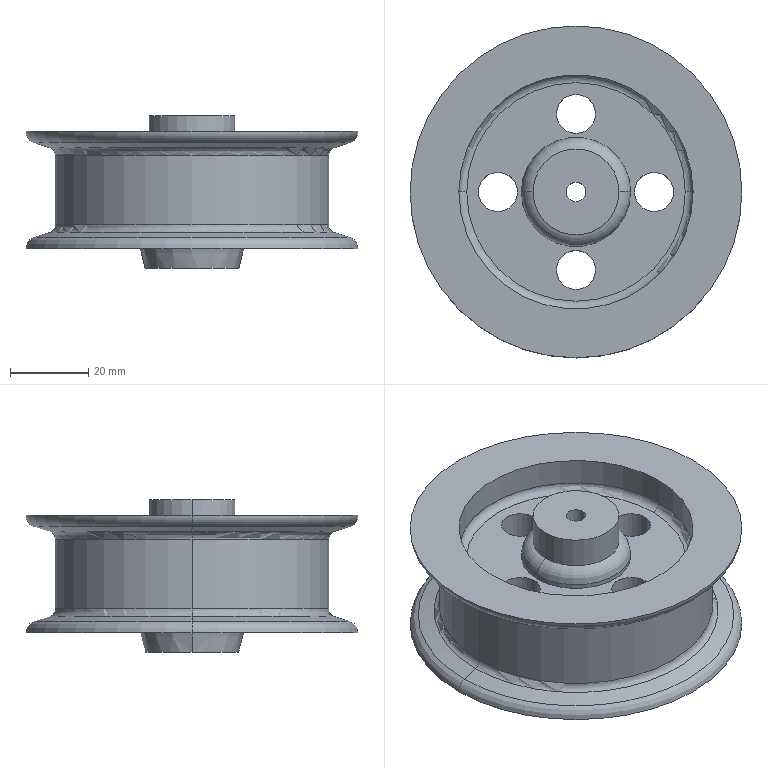Part | SolidWorks | features ICE 6, Fillet 2, Blend 1, Chamfer 1, Extrusion 1, HoleWzd 1, RevCut 1 | 1 solid | 46 faces | box 85 x 85 x 39 mm | volume 97267 mm3 | cylinder 20 | torus 12 | cone 8 | plane 6 | commonest cylinder face diameters 10 x8 60 x4 5 x2 22 x2 28 x2 70 x2
STEP:
#1=CARTESIAN_POINT('',(-12.,0.,-20.));
#2=VERTEX_POINT('',#1);
#3=CARTESIAN_POINT('',(12.,0.,-20.));
#4=VERTEX_POINT('',#3);
#5=CARTESIAN_POINT('',(0.,0.,-20.));
#6=DIRECTION('',(0.,0.,-1.));
#7=DIRECTION('',(-1.,0.,0.));
#8=AXIS2_PLACEMENT_3D('',#5,#6,#7);
#9=CIRCLE('',#8,12.);
#10=EDGE_CURVE('',#2,#4,#9,.T.);
#11=ORIENTED_EDGE('',*,*,#10,.F.);
#12=CARTESIAN_POINT('',(-14.,0.,-12.));
#13=VERTEX_POINT('',#12);
#14=CARTESIAN_POINT('',(-12.,0.,-20.));
#15=DIRECTION('',(-0.2425,0.,0.9701));
#16=VECTOR('',#15,1000.);
#17=LINE('',#14,#16);
#18=EDGE_CURVE('',#2,#13,#17,.T.);
#19=ORIENTED_EDGE('',*,*,#18,.T.);
#20=CARTESIAN_POINT('',(14.,0.,-12.));
#21=VERTEX_POINT('',#20);
#22=CARTESIAN_POINT('',(0.,0.,-12.));
#23=DIRECTION('',(0.,0.,-1.));
#24=DIRECTION('',(-1.,0.,0.));
#25=AXIS2_PLACEMENT_3D('',#22,#23,#24);
#26=CIRCLE('',#25,14.);
#27=EDGE_CURVE('',#13,#21,#26,.T.);
#28=ORIENTED_EDGE('',*,*,#27,.T.);
#29=CARTESIAN_POINT('',(12.,0.,-20.));
#30=DIRECTION('',(0.2425,0.,0.9701));
#31=VECTOR('',#30,1000.);
#32=LINE('',#29,#31);
#33=EDGE_CURVE('',#4,#21,#32,.T.);
#34=ORIENTED_EDGE('',*,*,#33,.F.);
#35=EDGE_LOOP('',(#11,#19,#28,#34));
#36=FACE_OUTER_BOUND('',#35,.T.);
#37=CARTESIAN_POINT('',(0.,0.,-20.));
#38=DIRECTION('',(0.,0.,1.));
#39=DIRECTION('',(1.,0.,0.));
#40=AXIS2_PLACEMENT_3D('',#37,#38,#39);
#41=CONICAL_SURFACE('',#40,12.,0.245);
#42=ADVANCED_FACE('',(#36),#41,.T.);
#43=CARTESIAN_POINT('',(2.5,0.,-20.));
#44=VERTEX_POINT('',#43);
#45=CARTESIAN_POINT('',(-2.5,0.,-20.));
#46=VERTEX_POINT('',#45);
#47=CARTESIAN_POINT('',(0.,0.,-20.));
#48=DIRECTION('',(0.,0.,-1.));
#49=DIRECTION('',(-1.,0.,0.));
#50=AXIS2_PLACEMENT_3D('',#47,#48,#49);
#51=CIRCLE('',#50,2.5);
#52=EDGE_CURVE('',#44,#46,#51,.T.);
#53=ORIENTED_EDGE('',*,*,#52,.T.);
#54=CARTESIAN_POINT('',(-2.5,0.,19.));
#55=VERTEX_POINT('',#54);
#56=CARTESIAN_POINT('',(-2.5,0.,19.));
#57=DIRECTION('',(0.,0.,1.));
#58=VECTOR('',#57,1000.);
#59=LINE('',#56,#58);
#60=EDGE_CURVE('',#46,#55,#59,.T.);
#61=ORIENTED_EDGE('',*,*,#60,.T.);
#62=CARTESIAN_POINT('',(2.5,0.,19.));
#63=VERTEX_POINT('',#62);
#64=CARTESIAN_POINT('',(0.,0.,19.));
#65=DIRECTION('',(0.,0.,1.));
#66=DIRECTION('',(1.,0.,0.));
#67=AXIS2_PLACEMENT_3D('',#64,#65,#66);
#68=CIRCLE('',#67,2.5);
#69=EDGE_CURVE('',#55,#63,#68,.T.);
#70=ORIENTED_EDGE('',*,*,#69,.T.);
#71=CARTESIAN_POINT('',(2.5,0.,19.));
#72=DIRECTION('',(0.,0.,1.));
#73=VECTOR('',#72,1000.);
#74=LINE('',#71,#73);
#75=EDGE_CURVE('',#44,#63,#74,.T.);
#76=ORIENTED_EDGE('',*,*,#75,.F.);
#77=EDGE_LOOP('',(#53,#61,#70,#76));
#78=FACE_OUTER_BOUND('',#77,.T.);
#79=CARTESIAN_POINT('',(0.,0.,19.));
#80=DIRECTION('',(0.,0.,1.));
#81=DIRECTION('',(1.,0.,0.));
#82=AXIS2_PLACEMENT_3D('',#79,#80,#81);
#83=CYLINDRICAL_SURFACE('',#82,2.5);
#84=ADVANCED_FACE('',(#78),#83,.F.);
#85=CARTESIAN_POINT('',(-36.382,0.,-10.833));
#86=VERTEX_POINT('',#85);
#87=CARTESIAN_POINT('',(36.382,0.,-10.833));
#88=VERTEX_POINT('',#87);
#89=CARTESIAN_POINT('',(0.,0.,-10.833));
#90=DIRECTION('',(0.,0.,-1.));
#91=DIRECTION('',(-1.,0.,0.));
#92=AXIS2_PLACEMENT_3D('',#89,#90,#91);
#93=CIRCLE('',#92,36.382);
#94=EDGE_CURVE('',#86,#88,#93,.T.);
#95=ORIENTED_EDGE('',*,*,#94,.T.);
#96=CARTESIAN_POINT('',(40.427,0.,-12.147));
#97=VERTEX_POINT('',#96);
#98=CARTESIAN_POINT('',(40.427,0.,-12.147));
#99=DIRECTION('',(0.9511,0.,-0.309));
#100=VECTOR('',#99,1000.);
#101=LINE('',#98,#100);
#102=EDGE_CURVE('',#88,#97,#101,.T.);
#103=ORIENTED_EDGE('',*,*,#102,.T.);
#104=CARTESIAN_POINT('',(-40.427,0.,-12.147));
#105=VERTEX_POINT('',#104);
#106=CARTESIAN_POINT('',(0.,0.,-12.147));
#107=DIRECTION('',(0.,0.,-1.));
#108=DIRECTION('',(-1.,0.,0.));
#109=AXIS2_PLACEMENT_3D('',#106,#107,#108);
#110=CIRCLE('',#109,40.427);
#111=EDGE_CURVE('',#105,#97,#110,.T.);
#112=ORIENTED_EDGE('',*,*,#111,.F.);
#113=CARTESIAN_POINT('',(-40.427,0.,-12.147));
#114=DIRECTION('',(-0.9511,0.,-0.309));
#115=VECTOR('',#114,1000.);
#116=LINE('',#113,#115);
#117=EDGE_CURVE('',#86,#105,#116,.T.);
#118=ORIENTED_EDGE('',*,*,#117,.F.);
#119=EDGE_LOOP('',(#95,#103,#112,#118));
#120=FACE_OUTER_BOUND('',#119,.T.);
#121=CARTESIAN_POINT('',(0.,0.,-12.147));
#122=DIRECTION('',(0.,0.,-1.));
#123=DIRECTION('',(-1.,0.,0.));
#124=AXIS2_PLACEMENT_3D('',#121,#122,#123);
#125=CONICAL_SURFACE('',#124,40.427,1.257);
#126=ADVANCED_FACE('',(#120),#125,.T.);
#127=CARTESIAN_POINT('',(0.,0.,-10.833));
#128=DIRECTION('',(0.,0.,-1.));
#129=DIRECTION('',(-1.,0.,0.));
#130=AXIS2_PLACEMENT_3D('',#127,#128,#129);
#131=CIRCLE('',#130,36.382);
#132=EDGE_CURVE('',#88,#86,#131,.T.);
#133=ORIENTED_EDGE('',*,*,#132,.F.);
#134=CARTESIAN_POINT('',(35.,0.,-8.93));
#135=VERTEX_POINT('',#134);
#136=CARTESIAN_POINT('',(37.,0.,-8.93));
#137=DIRECTION('',(0.,1.,0.));
#138=DIRECTION('',(-1.,0.,0.));
#139=AXIS2_PLACEMENT_3D('',#136,#137,#138);
#140=CIRCLE('',#139,2.);
#141=EDGE_CURVE('',#88,#135,#140,.T.);
#142=ORIENTED_EDGE('',*,*,#141,.T.);
#143=CARTESIAN_POINT('',(-35.,0.,-8.93));
#144=VERTEX_POINT('',#143);
#145=CARTESIAN_POINT('',(0.,0.,-8.93));
#146=DIRECTION('',(0.,0.,-1.));
#147=DIRECTION('',(-1.,0.,0.));
#148=AXIS2_PLACEMENT_3D('',#145,#146,#147);
#149=CIRCLE('',#148,35.);
#150=EDGE_CURVE('',#135,#144,#149,.T.);
#151=ORIENTED_EDGE('',*,*,#150,.T.);
#152=CARTESIAN_POINT('',(-37.,0.,-8.93));
#153=DIRECTION('',(0.,-1.,0.));
#154=DIRECTION('',(0.,0.,-1.));
#155=AXIS2_PLACEMENT_3D('',#152,#153,#154);
#156=CIRCLE('',#155,2.);
#157=EDGE_CURVE('',#86,#144,#156,.T.);
#158=ORIENTED_EDGE('',*,*,#157,.F.);
#159=EDGE_LOOP('',(#133,#142,#151,#158));
#160=FACE_OUTER_BOUND('',#159,.T.);
#161=CARTESIAN_POINT('',(0.,0.,-8.93));
#162=DIRECTION('',(0.,0.,-1.));
#163=DIRECTION('',(-1.,0.,0.));
#164=AXIS2_PLACEMENT_3D('',#161,#162,#163);
#165=TOROIDAL_SURFACE('',#164,37.,2.);
#166=ADVANCED_FACE('',(#160),#165,.F.);
#167=CARTESIAN_POINT('',(-35.,0.,8.93));
#168=VERTEX_POINT('',#167);
#169=CARTESIAN_POINT('',(35.,0.,8.93));
#170=VERTEX_POINT('',#169);
#171=CARTESIAN_POINT('',(0.,0.,8.93));
#172=DIRECTION('',(0.,0.,-1.));
#173=DIRECTION('',(-1.,0.,0.));
#174=AXIS2_PLACEMENT_3D('',#171,#172,#173);
#175=CIRCLE('',#174,35.);
#176=EDGE_CURVE('',#168,#170,#175,.T.);
#177=ORIENTED_EDGE('',*,*,#176,.T.);
#178=CARTESIAN_POINT('',(35.,0.,0.));
#179=DIRECTION('',(0.,0.,-1.));
#180=VECTOR('',#179,1000.);
#181=LINE('',#178,#180);
#182=EDGE_CURVE('',#170,#135,#181,.T.);
#183=ORIENTED_EDGE('',*,*,#182,.T.);
#184=CARTESIAN_POINT('',(0.,0.,-8.93));
#185=DIRECTION('',(0.,0.,-1.));
#186=DIRECTION('',(-1.,0.,0.));
#187=AXIS2_PLACEMENT_3D('',#184,#185,#186);
#188=CIRCLE('',#187,35.);
#189=EDGE_CURVE('',#144,#135,#188,.T.);
#190=ORIENTED_EDGE('',*,*,#189,.F.);
#191=CARTESIAN_POINT('',(-35.,0.,0.));
#192=DIRECTION('',(0.,0.,-1.));
#193=VECTOR('',#192,1000.);
#194=LINE('',#191,#193);
#195=EDGE_CURVE('',#168,#144,#194,.T.);
#196=ORIENTED_EDGE('',*,*,#195,.F.);
#197=EDGE_LOOP('',(#177,#183,#190,#196));
#198=FACE_OUTER_BOUND('',#197,.T.);
#199=CARTESIAN_POINT('',(0.,0.,0.));
#200=DIRECTION('',(0.,0.,-1.));
#201=DIRECTION('',(-1.,0.,0.));
#202=AXIS2_PLACEMENT_3D('',#199,#200,#201);
#203=CYLINDRICAL_SURFACE('',#202,35.);
#204=ADVANCED_FACE('',(#198),#203,.T.);
#205=CARTESIAN_POINT('',(0.,0.,8.93));
#206=DIRECTION('',(0.,0.,-1.));
#207=DIRECTION('',(-1.,0.,0.));
#208=AXIS2_PLACEMENT_3D('',#205,#206,#207);
#209=CIRCLE('',#208,35.);
#210=EDGE_CURVE('',#170,#168,#209,.T.);
#211=ORIENTED_EDGE('',*,*,#210,.F.);
#212=CARTESIAN_POINT('',(36.382,0.,10.833));
#213=VERTEX_POINT('',#212);
#214=CARTESIAN_POINT('',(37.,0.,8.93));
#215=DIRECTION('',(0.,1.,0.));
#216=DIRECTION('',(-1.,0.,0.));
#217=AXIS2_PLACEMENT_3D('',#214,#215,#216);
#218=CIRCLE('',#217,2.);
#219=EDGE_CURVE('',#170,#213,#218,.T.);
#220=ORIENTED_EDGE('',*,*,#219,.T.);
#221=CARTESIAN_POINT('',(-36.382,0.,10.833));
#222=VERTEX_POINT('',#221);
#223=CARTESIAN_POINT('',(0.,0.,10.833));
#224=DIRECTION('',(0.,0.,-1.));
#225=DIRECTION('',(-1.,0.,0.));
#226=AXIS2_PLACEMENT_3D('',#223,#224,#225);
#227=CIRCLE('',#226,36.382);
#228=EDGE_CURVE('',#213,#222,#227,.T.);
#229=ORIENTED_EDGE('',*,*,#228,.T.);
#230=CARTESIAN_POINT('',(-37.,0.,8.93));
#231=DIRECTION('',(0.,-1.,0.));
#232=DIRECTION('',(0.,0.,-1.));
#233=AXIS2_PLACEMENT_3D('',#230,#231,#232);
#234=CIRCLE('',#233,2.);
#235=EDGE_CURVE('',#168,#222,#234,.T.);
#236=ORIENTED_EDGE('',*,*,#235,.F.);
#237=EDGE_LOOP('',(#211,#220,#229,#236));
#238=FACE_OUTER_BOUND('',#237,.T.);
#239=CARTESIAN_POINT('',(0.,0.,8.93));
#240=DIRECTION('',(0.,0.,-1.));
#241=DIRECTION('',(-1.,0.,0.));
#242=AXIS2_PLACEMENT_3D('',#239,#240,#241);
#243=TOROIDAL_SURFACE('',#242,37.,2.);
#244=ADVANCED_FACE('',(#238),#243,.F.);
#245=CARTESIAN_POINT('',(0.,0.,10.833));
#246=DIRECTION('',(0.,0.,-1.));
#247=DIRECTION('',(-1.,0.,0.));
#248=AXIS2_PLACEMENT_3D('',#245,#246,#247);
#249=CIRCLE('',#248,36.382);
#250=EDGE_CURVE('',#222,#213,#249,.T.);
#251=ORIENTED_EDGE('',*,*,#250,.F.);
#252=CARTESIAN_POINT('',(-40.427,0.,12.147));
#253=VERTEX_POINT('',#252);
#254=CARTESIAN_POINT('',(-36.382,0.,10.833));
#255=DIRECTION('',(-0.9511,0.,0.309));
#256=VECTOR('',#255,1000.);
#257=LINE('',#254,#256);
#258=EDGE_CURVE('',#222,#253,#257,.T.);
#259=ORIENTED_EDGE('',*,*,#258,.T.);
#260=CARTESIAN_POINT('',(40.427,0.,12.147));
#261=VERTEX_POINT('',#260);
#262=CARTESIAN_POINT('',(0.,0.,12.147));
#263=DIRECTION('',(0.,0.,-1.));
#264=DIRECTION('',(-1.,0.,0.));
#265=AXIS2_PLACEMENT_3D('',#262,#263,#264);
#266=CIRCLE('',#265,40.427);
#267=EDGE_CURVE('',#253,#261,#266,.T.);
#268=ORIENTED_EDGE('',*,*,#267,.T.);
#269=CARTESIAN_POINT('',(36.382,0.,10.833));
#270=DIRECTION('',(0.9511,0.,0.309));
#271=VECTOR('',#270,1000.);
#272=LINE('',#269,#271);
#273=EDGE_CURVE('',#213,#261,#272,.T.);
#274=ORIENTED_EDGE('',*,*,#273,.F.);
#275=EDGE_LOOP('',(#251,#259,#268,#274));
#276=FACE_OUTER_BOUND('',#275,.T.);
#277=CARTESIAN_POINT('',(0.,0.,10.833));
#278=DIRECTION('',(0.,0.,1.));
#279=DIRECTION('',(1.,0.,0.));
#280=AXIS2_PLACEMENT_3D('',#277,#278,#279);
#281=CONICAL_SURFACE('',#280,36.382,1.257);
#282=ADVANCED_FACE('',(#276),#281,.T.);
#283=CARTESIAN_POINT('',(-42.5,0.,15.));
#284=VERTEX_POINT('',#283);
#285=CARTESIAN_POINT('',(42.5,0.,15.));
#286=VERTEX_POINT('',#285);
#287=CARTESIAN_POINT('',(0.,0.,15.));
#288=DIRECTION('',(0.,0.,-1.));
#289=DIRECTION('',(-1.,0.,0.));
#290=AXIS2_PLACEMENT_3D('',#287,#288,#289);
#291=CIRCLE('',#290,42.5);
#292=EDGE_CURVE('',#284,#286,#291,.T.);
#293=ORIENTED_EDGE('',*,*,#292,.T.);
#294=CARTESIAN_POINT('',(39.5,0.,15.));
#295=DIRECTION('',(0.,1.,0.));
#296=DIRECTION('',(-1.,0.,0.));
#297=AXIS2_PLACEMENT_3D('',#294,#295,#296);
#298=CIRCLE('',#297,3.);
#299=EDGE_CURVE('',#286,#261,#298,.T.);
#300=ORIENTED_EDGE('',*,*,#299,.T.);
#301=ORIENTED_EDGE('',*,*,#267,.F.);
#302=CARTESIAN_POINT('',(-39.5,0.,15.));
#303=DIRECTION('',(0.,-1.,0.));
#304=DIRECTION('',(0.,0.,-1.));
#305=AXIS2_PLACEMENT_3D('',#302,#303,#304);
#306=CIRCLE('',#305,3.);
#307=EDGE_CURVE('',#284,#253,#306,.T.);
#308=ORIENTED_EDGE('',*,*,#307,.F.);
#309=EDGE_LOOP('',(#293,#300,#301,#308));
#310=FACE_OUTER_BOUND('',#309,.T.);
#311=CARTESIAN_POINT('',(0.,0.,15.));
#312=DIRECTION('',(0.,0.,-1.));
#313=DIRECTION('',(-1.,0.,0.));
#314=AXIS2_PLACEMENT_3D('',#311,#312,#313);
#315=TOROIDAL_SURFACE('',#314,39.5,3.);
#316=ADVANCED_FACE('',(#310),#315,.T.);
#317=ORIENTED_EDGE('',*,*,#111,.T.);
#318=CARTESIAN_POINT('',(42.5,0.,-15.));
#319=VERTEX_POINT('',#318);
#320=CARTESIAN_POINT('',(39.5,0.,-15.));
#321=DIRECTION('',(0.,1.,0.));
#322=DIRECTION('',(-1.,0.,0.));
#323=AXIS2_PLACEMENT_3D('',#320,#321,#322);
#324=CIRCLE('',#323,3.);
#325=EDGE_CURVE('',#97,#319,#324,.T.);
#326=ORIENTED_EDGE('',*,*,#325,.T.);
#327=CARTESIAN_POINT('',(-42.5,0.,-15.));
#328=VERTEX_POINT('',#327);
#329=CARTESIAN_POINT('',(0.,0.,-15.));
#330=DIRECTION('',(0.,0.,-1.));
#331=DIRECTION('',(-1.,0.,0.));
#332=AXIS2_PLACEMENT_3D('',#329,#330,#331);
#333=CIRCLE('',#332,42.5);
#334=EDGE_CURVE('',#328,#319,#333,.T.);
#335=ORIENTED_EDGE('',*,*,#334,.F.);
#336=CARTESIAN_POINT('',(-39.5,0.,-15.));
#337=DIRECTION('',(0.,-1.,0.));
#338=DIRECTION('',(0.,0.,-1.));
#339=AXIS2_PLACEMENT_3D('',#336,#337,#338);
#340=CIRCLE('',#339,3.);
#341=EDGE_CURVE('',#105,#328,#340,.T.);
#342=ORIENTED_EDGE('',*,*,#341,.F.);
#343=EDGE_LOOP('',(#317,#326,#335,#342));
#344=FACE_OUTER_BOUND('',#343,.T.);
#345=CARTESIAN_POINT('',(0.,0.,-15.));
#346=DIRECTION('',(0.,0.,-1.));
#347=DIRECTION('',(-1.,0.,0.));
#348=AXIS2_PLACEMENT_3D('',#345,#346,#347);
#349=TOROIDAL_SURFACE('',#348,39.5,3.);
#350=ADVANCED_FACE('',(#344),#349,.T.);
#351=CARTESIAN_POINT('',(30.,0.,-14.));
#352=VERTEX_POINT('',#351);
#353=CARTESIAN_POINT('',(-30.,0.,-14.));
#354=VERTEX_POINT('',#353);
#355=CARTESIAN_POINT('',(0.,0.,-14.));
#356=DIRECTION('',(0.,0.,-1.));
#357=DIRECTION('',(1.,0.,0.));
#358=AXIS2_PLACEMENT_3D('',#355,#356,#357);
#359=CIRCLE('',#358,30.);
#360=EDGE_CURVE('',#352,#354,#359,.T.);
#361=ORIENTED_EDGE('',*,*,#360,.F.);
#362=CARTESIAN_POINT('',(31.,0.,-15.));
#363=VERTEX_POINT('',#362);
#364=CARTESIAN_POINT('',(31.,0.,-15.));
#365=DIRECTION('',(0.7071,0.,-0.7071));
#366=VECTOR('',#365,1000.);
#367=LINE('',#364,#366);
#368=EDGE_CURVE('',#352,#363,#367,.T.);
#369=ORIENTED_EDGE('',*,*,#368,.T.);
#370=CARTESIAN_POINT('',(-31.,0.,-15.));
#371=VERTEX_POINT('',#370);
#372=CARTESIAN_POINT('',(0.,0.,-15.));
#373=DIRECTION('',(0.,0.,1.));
#374=DIRECTION('',(1.,0.,0.));
#375=AXIS2_PLACEMENT_3D('',#372,#373,#374);
#376=CIRCLE('',#375,31.);
#377=EDGE_CURVE('',#371,#363,#376,.T.);
#378=ORIENTED_EDGE('',*,*,#377,.F.);
#379=CARTESIAN_POINT('',(-31.,0.,-15.));
#380=DIRECTION('',(-0.7071,0.,-0.7071));
#381=VECTOR('',#380,1000.);
#382=LINE('',#379,#381);
#383=EDGE_CURVE('',#354,#371,#382,.T.);
#384=ORIENTED_EDGE('',*,*,#383,.F.);
#385=EDGE_LOOP('',(#361,#369,#378,#384));
#386=FACE_OUTER_BOUND('',#385,.T.);
#387=CARTESIAN_POINT('',(0.,0.,-15.));
#388=DIRECTION('',(0.,0.,-1.));
#389=DIRECTION('',(-1.,0.,0.));
#390=AXIS2_PLACEMENT_3D('',#387,#388,#389);
#391=CONICAL_SURFACE('',#390,31.,0.7854);
#392=ADVANCED_FACE('',(#386),#391,.F.);
#393=CARTESIAN_POINT('',(-14.,0.,7.127));
#394=VERTEX_POINT('',#393);
#395=CARTESIAN_POINT('',(14.,0.,7.127));
#396=VERTEX_POINT('',#395);
#397=CARTESIAN_POINT('',(0.,0.,7.127));
#398=DIRECTION('',(0.,0.,-1.));
#399=DIRECTION('',(1.,0.,0.));
#400=AXIS2_PLACEMENT_3D('',#397,#398,#399);
#401=CIRCLE('',#400,14.);
#402=EDGE_CURVE('',#394,#396,#401,.T.);
#403=ORIENTED_EDGE('',*,*,#402,.F.);
#404=CARTESIAN_POINT('',(-11.,0.,11.));
#405=VERTEX_POINT('',#404);
#406=CARTESIAN_POINT('',(-10.,0.,7.127));
#407=DIRECTION('',(0.,1.,0.));
#408=DIRECTION('',(-1.,0.,0.));
#409=AXIS2_PLACEMENT_3D('',#406,#407,#408);
#410=CIRCLE('',#409,4.);
#411=EDGE_CURVE('',#394,#405,#410,.T.);
#412=ORIENTED_EDGE('',*,*,#411,.T.);
#413=CARTESIAN_POINT('',(11.,0.,11.));
#414=VERTEX_POINT('',#413);
#415=CARTESIAN_POINT('',(0.,0.,11.));
#416=DIRECTION('',(0.,0.,1.));
#417=DIRECTION('',(1.,0.,0.));
#418=AXIS2_PLACEMENT_3D('',#415,#416,#417);
#419=CIRCLE('',#418,11.);
#420=EDGE_CURVE('',#414,#405,#419,.T.);
#421=ORIENTED_EDGE('',*,*,#420,.F.);
#422=CARTESIAN_POINT('',(10.,0.,7.127));
#423=DIRECTION('',(0.,-1.,0.));
#424=DIRECTION('',(0.,0.,-1.));
#425=AXIS2_PLACEMENT_3D('',#422,#423,#424);
#426=CIRCLE('',#425,4.);
#427=EDGE_CURVE('',#396,#414,#426,.T.);
#428=ORIENTED_EDGE('',*,*,#427,.F.);
#429=EDGE_LOOP('',(#403,#412,#421,#428));
#430=FACE_OUTER_BOUND('',#429,.T.);
#431=CARTESIAN_POINT('',(0.,0.,7.127));
#432=DIRECTION('',(0.,0.,1.));
#433=DIRECTION('',(1.,0.,0.));
#434=AXIS2_PLACEMENT_3D('',#431,#432,#433);
#435=TOROIDAL_SURFACE('',#434,10.,4.);
#436=ADVANCED_FACE('',(#430),#435,.T.);
#437=CARTESIAN_POINT('',(11.,0.,19.));
#438=VERTEX_POINT('',#437);
#439=CARTESIAN_POINT('',(-11.,0.,19.));
#440=VERTEX_POINT('',#439);
#441=CARTESIAN_POINT('',(0.,0.,19.));
#442=DIRECTION('',(0.,0.,1.));
#443=DIRECTION('',(1.,0.,0.));
#444=AXIS2_PLACEMENT_3D('',#441,#442,#443);
#445=CIRCLE('',#444,11.);
#446=EDGE_CURVE('',#438,#440,#445,.T.);
#447=ORIENTED_EDGE('',*,*,#446,.F.);
#448=CARTESIAN_POINT('',(11.,0.,19.));
#449=DIRECTION('',(0.,0.,-1.));
#450=VECTOR('',#449,1000.);
#451=LINE('',#448,#450);
#452=EDGE_CURVE('',#438,#414,#451,.T.);
#453=ORIENTED_EDGE('',*,*,#452,.T.);
#454=ORIENTED_EDGE('',*,*,#420,.T.);
#455=CARTESIAN_POINT('',(-11.,0.,19.));
#456=DIRECTION('',(0.,0.,-1.));
#457=VECTOR('',#456,1000.);
#458=LINE('',#455,#457);
#459=EDGE_CURVE('',#440,#405,#458,.T.);
#460=ORIENTED_EDGE('',*,*,#459,.F.);
#461=EDGE_LOOP('',(#447,#453,#454,#460));
#462=FACE_OUTER_BOUND('',#461,.T.);
#463=CARTESIAN_POINT('',(0.,0.,19.));
#464=DIRECTION('',(0.,0.,-1.));
#465=DIRECTION('',(-1.,0.,0.));
#466=AXIS2_PLACEMENT_3D('',#463,#464,#465);
#467=CYLINDRICAL_SURFACE('',#466,11.);
#468=ADVANCED_FACE('',(#462),#467,.T.);
#469=ORIENTED_EDGE('',*,*,#402,.T.);
#470=CARTESIAN_POINT('',(14.,0.,6.));
#471=VERTEX_POINT('',#470);
#472=CARTESIAN_POINT('',(14.,0.,11.));
#473=DIRECTION('',(0.,0.,-1.));
#474=VECTOR('',#473,1000.);
#475=LINE('',#472,#474);
#476=EDGE_CURVE('',#396,#471,#475,.T.);
#477=ORIENTED_EDGE('',*,*,#476,.T.);
#478=CARTESIAN_POINT('',(-14.,0.,6.));
#479=VERTEX_POINT('',#478);
#480=CARTESIAN_POINT('',(0.,0.,6.));
#481=DIRECTION('',(0.,0.,1.));
#482=DIRECTION('',(1.,0.,0.));
#483=AXIS2_PLACEMENT_3D('',#480,#481,#482);
#484=CIRCLE('',#483,14.);
#485=EDGE_CURVE('',#471,#479,#484,.T.);
#486=ORIENTED_EDGE('',*,*,#485,.T.);
#487=CARTESIAN_POINT('',(-14.,0.,11.));
#488=DIRECTION('',(0.,0.,-1.));
#489=VECTOR('',#488,1000.);
#490=LINE('',#487,#489);
#491=EDGE_CURVE('',#394,#479,#490,.T.);
#492=ORIENTED_EDGE('',*,*,#491,.F.);
#493=EDGE_LOOP('',(#469,#477,#486,#492));
#494=FACE_OUTER_BOUND('',#493,.T.);
#495=CARTESIAN_POINT('',(0.,0.,11.));
#496=DIRECTION('',(0.,0.,-1.));
#497=DIRECTION('',(-1.,0.,0.));
#498=AXIS2_PLACEMENT_3D('',#495,#496,#497);
#499=CYLINDRICAL_SURFACE('',#498,14.);
#500=ADVANCED_FACE('',(#494),#499,.T.);
#501=CARTESIAN_POINT('',(-28.,0.,6.));
#502=VERTEX_POINT('',#501);
#503=CARTESIAN_POINT('',(28.,0.,6.));
#504=VERTEX_POINT('',#503);
#505=CARTESIAN_POINT('',(0.,0.,6.));
#506=DIRECTION('',(0.,0.,1.));
#507=DIRECTION('',(1.,0.,0.));
#508=AXIS2_PLACEMENT_3D('',#505,#506,#507);
#509=CIRCLE('',#508,28.);
#510=EDGE_CURVE('',#502,#504,#509,.T.);
#511=ORIENTED_EDGE('',*,*,#510,.F.);
#512=CARTESIAN_POINT('',(-30.,0.,8.));
#513=VERTEX_POINT('',#512);
#514=CARTESIAN_POINT('',(-28.,0.,8.));
#515=DIRECTION('',(0.,1.,0.));
#516=DIRECTION('',(-1.,0.,0.));
#517=AXIS2_PLACEMENT_3D('',#514,#515,#516);
#518=CIRCLE('',#517,2.);
#519=EDGE_CURVE('',#502,#513,#518,.T.);
#520=ORIENTED_EDGE('',*,*,#519,.T.);
#521=CARTESIAN_POINT('',(30.,0.,8.));
#522=VERTEX_POINT('',#521);
#523=CARTESIAN_POINT('',(0.,0.,8.));
#524=DIRECTION('',(0.,0.,-1.));
#525=DIRECTION('',(1.,0.,0.));
#526=AXIS2_PLACEMENT_3D('',#523,#524,#525);
#527=CIRCLE('',#526,30.);
#528=EDGE_CURVE('',#522,#513,#527,.T.);
#529=ORIENTED_EDGE('',*,*,#528,.F.);
#530=CARTESIAN_POINT('',(28.,0.,8.));
#531=DIRECTION('',(0.,-1.,0.));
#532=DIRECTION('',(0.,0.,-1.));
#533=AXIS2_PLACEMENT_3D('',#530,#531,#532);
#534=CIRCLE('',#533,2.);
#535=EDGE_CURVE('',#504,#522,#534,.T.);
#536=ORIENTED_EDGE('',*,*,#535,.F.);
#537=EDGE_LOOP('',(#511,#520,#529,#536));
#538=FACE_OUTER_BOUND('',#537,.T.);
#539=CARTESIAN_POINT('',(0.,0.,8.));
#540=DIRECTION('',(0.,0.,1.));
#541=DIRECTION('',(1.,0.,0.));
#542=AXIS2_PLACEMENT_3D('',#539,#540,#541);
#543=TOROIDAL_SURFACE('',#542,28.,2.);
#544=ADVANCED_FACE('',(#538),#543,.F.);
#545=CARTESIAN_POINT('',(5.,20.,-12.));
#546=VERTEX_POINT('',#545);
#547=CARTESIAN_POINT('',(-5.,20.,-12.));
#548=VERTEX_POINT('',#547);
#549=CARTESIAN_POINT('',(0.,20.,-12.));
#550=DIRECTION('',(0.,0.,-1.));
#551=DIRECTION('',(-1.,0.,0.));
#552=AXIS2_PLACEMENT_3D('',#549,#550,#551);
#553=CIRCLE('',#552,5.);
#554=EDGE_CURVE('',#546,#548,#553,.T.);
#555=ORIENTED_EDGE('',*,*,#554,.T.);
#556=CARTESIAN_POINT('',(-5.,20.,6.));
#557=VERTEX_POINT('',#556);
#558=CARTESIAN_POINT('',(-5.,20.,-15.));
#559=DIRECTION('',(0.,0.,1.));
#560=VECTOR('',#559,1000.);
#561=LINE('',#558,#560);
#562=EDGE_CURVE('',#548,#557,#561,.T.);
#563=ORIENTED_EDGE('',*,*,#562,.T.);
#564=CARTESIAN_POINT('',(5.,20.,6.));
#565=VERTEX_POINT('',#564);
#566=CARTESIAN_POINT('',(0.,20.,6.));
#567=DIRECTION('',(0.,0.,1.));
#568=DIRECTION('',(1.,0.,0.));
#569=AXIS2_PLACEMENT_3D('',#566,#567,#568);
#570=CIRCLE('',#569,5.);
#571=EDGE_CURVE('',#557,#565,#570,.T.);
#572=ORIENTED_EDGE('',*,*,#571,.T.);
#573=CARTESIAN_POINT('',(5.,20.,-15.));
#574=DIRECTION('',(0.,0.,1.));
#575=VECTOR('',#574,1000.);
#576=LINE('',#573,#575);
#577=EDGE_CURVE('',#546,#565,#576,.T.);
#578=ORIENTED_EDGE('',*,*,#577,.F.);
#579=EDGE_LOOP('',(#555,#563,#572,#578));
#580=FACE_OUTER_BOUND('',#579,.T.);
#581=CARTESIAN_POINT('',(0.,20.,-15.));
#582=DIRECTION('',(0.,0.,1.));
#583=DIRECTION('',(1.,0.,0.));
#584=AXIS2_PLACEMENT_3D('',#581,#582,#583);
#585=CYLINDRICAL_SURFACE('',#584,5.);
#586=ADVANCED_FACE('',(#580),#585,.F.);
#587=CARTESIAN_POINT('',(25.,0.,-12.));
#588=VERTEX_POINT('',#587);
#589=CARTESIAN_POINT('',(15.,0.,-12.));
#590=VERTEX_POINT('',#589);
#591=CARTESIAN_POINT('',(20.,0.,-12.));
#592=DIRECTION('',(0.,0.,-1.));
#593=DIRECTION('',(-1.,0.,0.));
#594=AXIS2_PLACEMENT_3D('',#591,#592,#593);
#595=CIRCLE('',#594,5.);
#596=EDGE_CURVE('',#588,#590,#595,.T.);
#597=ORIENTED_EDGE('',*,*,#596,.T.);
#598=CARTESIAN_POINT('',(15.,0.,6.));
#599=VERTEX_POINT('',#598);
#600=CARTESIAN_POINT('',(15.,0.,-15.));
#601=DIRECTION('',(0.,0.,1.));
#602=VECTOR('',#601,1000.);
#603=LINE('',#600,#602);
#604=EDGE_CURVE('',#590,#599,#603,.T.);
#605=ORIENTED_EDGE('',*,*,#604,.T.);
#606=CARTESIAN_POINT('',(25.,0.,6.));
#607=VERTEX_POINT('',#606);
#608=CARTESIAN_POINT('',(20.,0.,6.));
#609=DIRECTION('',(0.,0.,1.));
#610=DIRECTION('',(1.,0.,0.));
#611=AXIS2_PLACEMENT_3D('',#608,#609,#610);
#612=CIRCLE('',#611,5.);
#613=EDGE_CURVE('',#599,#607,#612,.T.);
#614=ORIENTED_EDGE('',*,*,#613,.T.);
#615=CARTESIAN_POINT('',(25.,0.,-15.));
#616=DIRECTION('',(0.,0.,1.));
#617=VECTOR('',#616,1000.);
#618=LINE('',#615,#617);
#619=EDGE_CURVE('',#588,#607,#618,.T.);
#620=ORIENTED_EDGE('',*,*,#619,.F.);
#621=EDGE_LOOP('',(#597,#605,#614,#620));
#622=FACE_OUTER_BOUND('',#621,.T.);
#623=CARTESIAN_POINT('',(20.,0.,-15.));
#624=DIRECTION('',(0.,0.,1.));
#625=DIRECTION('',(1.,0.,0.));
#626=AXIS2_PLACEMENT_3D('',#623,#624,#625);
#627=CYLINDRICAL_SURFACE('',#626,5.);
#628=ADVANCED_FACE('',(#622),#627,.F.);
#629=CARTESIAN_POINT('',(5.,-20.,-12.));
#630=VERTEX_POINT('',#629);
#631=CARTESIAN_POINT('',(-5.,-20.,-12.));
#632=VERTEX_POINT('',#631);
#633=CARTESIAN_POINT('',(0.,-20.,-12.));
#634=DIRECTION('',(0.,0.,-1.));
#635=DIRECTION('',(-1.,0.,0.));
#636=AXIS2_PLACEMENT_3D('',#633,#634,#635);
#637=CIRCLE('',#636,5.);
#638=EDGE_CURVE('',#630,#632,#637,.T.);
#639=ORIENTED_EDGE('',*,*,#638,.T.);
#640=CARTESIAN_POINT('',(-5.,-20.,6.));
#641=VERTEX_POINT('',#640);
#642=CARTESIAN_POINT('',(-5.,-20.,-15.));
#643=DIRECTION('',(0.,0.,1.));
#644=VECTOR('',#643,1000.);
#645=LINE('',#642,#644);
#646=EDGE_CURVE('',#632,#641,#645,.T.);
#647=ORIENTED_EDGE('',*,*,#646,.T.);
#648=CARTESIAN_POINT('',(5.,-20.,6.));
#649=VERTEX_POINT('',#648);
#650=CARTESIAN_POINT('',(0.,-20.,6.));
#651=DIRECTION('',(0.,0.,1.));
#652=DIRECTION('',(1.,0.,0.));
#653=AXIS2_PLACEMENT_3D('',#650,#651,#652);
#654=CIRCLE('',#653,5.);
#655=EDGE_CURVE('',#641,#649,#654,.T.);
#656=ORIENTED_EDGE('',*,*,#655,.T.);
#657=CARTESIAN_POINT('',(5.,-20.,-15.));
#658=DIRECTION('',(0.,0.,1.));
#659=VECTOR('',#658,1000.);
#660=LINE('',#657,#659);
#661=EDGE_CURVE('',#630,#649,#660,.T.);
#662=ORIENTED_EDGE('',*,*,#661,.F.);
#663=EDGE_LOOP('',(#639,#647,#656,#662));
#664=FACE_OUTER_BOUND('',#663,.T.);
#665=CARTESIAN_POINT('',(0.,-20.,-15.));
#666=DIRECTION('',(0.,0.,1.));
#667=DIRECTION('',(1.,0.,0.));
#668=AXIS2_PLACEMENT_3D('',#665,#666,#667);
#669=CYLINDRICAL_SURFACE('',#668,5.);
#670=ADVANCED_FACE('',(#664),#669,.F.);
#671=CARTESIAN_POINT('',(-15.,0.,-12.));
#672=VERTEX_POINT('',#671);
#673=CARTESIAN_POINT('',(-25.,0.,-12.));
#674=VERTEX_POINT('',#673);
#675=CARTESIAN_POINT('',(-20.,0.,-12.));
#676=DIRECTION('',(0.,0.,-1.));
#677=DIRECTION('',(-1.,0.,0.));
#678=AXIS2_PLACEMENT_3D('',#675,#676,#677);
#679=CIRCLE('',#678,5.);
#680=EDGE_CURVE('',#672,#674,#679,.T.);
#681=ORIENTED_EDGE('',*,*,#680,.T.);
#682=CARTESIAN_POINT('',(-25.,0.,6.));
#683=VERTEX_POINT('',#682);
#684=CARTESIAN_POINT('',(-25.,0.,-15.));
#685=DIRECTION('',(0.,0.,1.));
#686=VECTOR('',#685,1000.);
#687=LINE('',#684,#686);
#688=EDGE_CURVE('',#674,#683,#687,.T.);
#689=ORIENTED_EDGE('',*,*,#688,.T.);
#690=CARTESIAN_POINT('',(-15.,0.,6.));
#691=VERTEX_POINT('',#690);
#692=CARTESIAN_POINT('',(-20.,0.,6.));
#693=DIRECTION('',(0.,0.,1.));
#694=DIRECTION('',(1.,0.,0.));
#695=AXIS2_PLACEMENT_3D('',#692,#693,#694);
#696=CIRCLE('',#695,5.);
#697=EDGE_CURVE('',#683,#691,#696,.T.);
#698=ORIENTED_EDGE('',*,*,#697,.T.);
#699=CARTESIAN_POINT('',(-15.,0.,-15.));
#700=DIRECTION('',(0.,0.,1.));
#701=VECTOR('',#700,1000.);
#702=LINE('',#699,#701);
#703=EDGE_CURVE('',#672,#691,#702,.T.);
#704=ORIENTED_EDGE('',*,*,#703,.F.);
#705=EDGE_LOOP('',(#681,#689,#698,#704));
#706=FACE_OUTER_BOUND('',#705,.T.);
#707=CARTESIAN_POINT('',(-20.,0.,-15.));
#708=DIRECTION('',(0.,0.,1.));
#709=DIRECTION('',(1.,0.,0.));
#710=AXIS2_PLACEMENT_3D('',#707,#708,#709);
#711=CYLINDRICAL_SURFACE('',#710,5.);
#712=ADVANCED_FACE('',(#706),#711,.F.);
#713=CARTESIAN_POINT('',(-30.,0.,15.));
#714=VERTEX_POINT('',#713);
#715=CARTESIAN_POINT('',(30.,0.,15.));
#716=VERTEX_POINT('',#715);
#717=CARTESIAN_POINT('',(0.,0.,15.));
#718=DIRECTION('',(0.,0.,1.));
#719=DIRECTION('',(1.,0.,0.));
#720=AXIS2_PLACEMENT_3D('',#717,#718,#719);
#721=CIRCLE('',#720,30.);
#722=EDGE_CURVE('',#714,#716,#721,.T.);
#723=ORIENTED_EDGE('',*,*,#722,.T.);
#724=CARTESIAN_POINT('',(30.,0.,15.));
#725=DIRECTION('',(0.,0.,-1.));
#726=VECTOR('',#725,1000.);
#727=LINE('',#724,#726);
#728=EDGE_CURVE('',#716,#522,#727,.T.);
#729=ORIENTED_EDGE('',*,*,#728,.T.);
#730=ORIENTED_EDGE('',*,*,#528,.T.);
#731=CARTESIAN_POINT('',(-30.,0.,15.));
#732=DIRECTION('',(0.,0.,-1.));
#733=VECTOR('',#732,1000.);
#734=LINE('',#731,#733);
#735=EDGE_CURVE('',#714,#513,#734,.T.);
#736=ORIENTED_EDGE('',*,*,#735,.F.);
#737=EDGE_LOOP('',(#723,#729,#730,#736));
#738=FACE_OUTER_BOUND('',#737,.T.);
#739=CARTESIAN_POINT('',(0.,0.,15.));
#740=DIRECTION('',(0.,0.,-1.));
#741=DIRECTION('',(-1.,0.,0.));
#742=AXIS2_PLACEMENT_3D('',#739,#740,#741);
#743=CYLINDRICAL_SURFACE('',#742,30.);
#744=ADVANCED_FACE('',(#738),#743,.F.);
#745=CARTESIAN_POINT('',(30.,0.,-12.));
#746=VERTEX_POINT('',#745);
#747=CARTESIAN_POINT('',(-30.,0.,-12.));
#748=VERTEX_POINT('',#747);
#749=CARTESIAN_POINT('',(0.,0.,-12.));
#750=DIRECTION('',(0.,0.,-1.));
#751=DIRECTION('',(-1.,0.,0.));
#752=AXIS2_PLACEMENT_3D('',#749,#750,#751);
#753=CIRCLE('',#752,30.);
#754=EDGE_CURVE('',#746,#748,#753,.T.);
#755=ORIENTED_EDGE('',*,*,#754,.F.);
#756=CARTESIAN_POINT('',(30.,0.,15.));
#757=DIRECTION('',(0.,0.,-1.));
#758=VECTOR('',#757,1000.);
#759=LINE('',#756,#758);
#760=EDGE_CURVE('',#746,#352,#759,.T.);
#761=ORIENTED_EDGE('',*,*,#760,.T.);
#762=ORIENTED_EDGE('',*,*,#360,.T.);
#763=CARTESIAN_POINT('',(-30.,0.,15.));
#764=DIRECTION('',(0.,0.,-1.));
#765=VECTOR('',#764,1000.);
#766=LINE('',#763,#765);
#767=EDGE_CURVE('',#748,#354,#766,.T.);
#768=ORIENTED_EDGE('',*,*,#767,.F.);
#769=EDGE_LOOP('',(#755,#761,#762,#768));
#770=FACE_OUTER_BOUND('',#769,.T.);
#771=CARTESIAN_POINT('',(0.,0.,15.));
#772=DIRECTION('',(0.,0.,-1.));
#773=DIRECTION('',(-1.,0.,0.));
#774=AXIS2_PLACEMENT_3D('',#771,#772,#773);
#775=CYLINDRICAL_SURFACE('',#774,30.);
#776=ADVANCED_FACE('',(#770),#775,.F.);
#777=ORIENTED_EDGE('',*,*,#596,.F.);
#778=CARTESIAN_POINT('',(20.,0.,-12.));
#779=DIRECTION('',(0.,0.,-1.));
#780=DIRECTION('',(-1.,0.,0.));
#781=AXIS2_PLACEMENT_3D('',#778,#779,#780);
#782=CIRCLE('',#781,5.);
#783=EDGE_CURVE('',#590,#588,#782,.T.);
#784=ORIENTED_EDGE('',*,*,#783,.F.);
#785=EDGE_LOOP('',(#777,#784));
#786=FACE_BOUND('',#785,.T.);
#787=ORIENTED_EDGE('',*,*,#680,.F.);
#788=CARTESIAN_POINT('',(-20.,0.,-12.));
#789=DIRECTION('',(0.,0.,-1.));
#790=DIRECTION('',(-1.,0.,0.));
#791=AXIS2_PLACEMENT_3D('',#788,#789,#790);
#792=CIRCLE('',#791,5.);
#793=EDGE_CURVE('',#674,#672,#792,.T.);
#794=ORIENTED_EDGE('',*,*,#793,.F.);
#795=EDGE_LOOP('',(#787,#794));
#796=FACE_BOUND('',#795,.T.);
#797=CARTESIAN_POINT('',(0.,0.,-12.));
#798=DIRECTION('',(0.,0.,-1.));
#799=DIRECTION('',(-1.,0.,0.));
#800=AXIS2_PLACEMENT_3D('',#797,#798,#799);
#801=CIRCLE('',#800,30.);
#802=EDGE_CURVE('',#748,#746,#801,.T.);
#803=ORIENTED_EDGE('',*,*,#802,.T.);
#804=ORIENTED_EDGE('',*,*,#754,.T.);
#805=EDGE_LOOP('',(#803,#804));
#806=FACE_OUTER_BOUND('',#805,.T.);
#807=ORIENTED_EDGE('',*,*,#638,.F.);
#808=CARTESIAN_POINT('',(0.,-20.,-12.));
#809=DIRECTION('',(0.,0.,-1.));
#810=DIRECTION('',(-1.,0.,0.));
#811=AXIS2_PLACEMENT_3D('',#808,#809,#810);
#812=CIRCLE('',#811,5.);
#813=EDGE_CURVE('',#632,#630,#812,.T.);
#814=ORIENTED_EDGE('',*,*,#813,.F.);
#815=EDGE_LOOP('',(#807,#814));
#816=FACE_BOUND('',#815,.T.);
#817=ORIENTED_EDGE('',*,*,#554,.F.);
#818=CARTESIAN_POINT('',(0.,20.,-12.));
#819=DIRECTION('',(0.,0.,-1.));
#820=DIRECTION('',(-1.,0.,0.));
#821=AXIS2_PLACEMENT_3D('',#818,#819,#820);
#822=CIRCLE('',#821,5.);
#823=EDGE_CURVE('',#548,#546,#822,.T.);
#824=ORIENTED_EDGE('',*,*,#823,.F.);
#825=EDGE_LOOP('',(#817,#824));
#826=FACE_BOUND('',#825,.T.);
#827=CARTESIAN_POINT('',(0.,0.,-12.));
#828=DIRECTION('',(0.,0.,-1.));
#829=DIRECTION('',(-1.,0.,0.));
#830=AXIS2_PLACEMENT_3D('',#827,#828,#829);
#831=CIRCLE('',#830,14.);
#832=EDGE_CURVE('',#21,#13,#831,.T.);
#833=ORIENTED_EDGE('',*,*,#832,.F.);
#834=ORIENTED_EDGE('',*,*,#27,.F.);
#835=EDGE_LOOP('',(#833,#834));
#836=FACE_BOUND('',#835,.T.);
#837=CARTESIAN_POINT('',(0.,0.,-12.));
#838=DIRECTION('',(0.,0.,-1.));
#839=DIRECTION('',(-1.,0.,0.));
#840=AXIS2_PLACEMENT_3D('',#837,#838,#839);
#841=PLANE('',#840);
#842=ADVANCED_FACE('',(#786,#796,#806,#816,#826,#836),#841,.T.);
#843=ORIENTED_EDGE('',*,*,#760,.F.);
#844=ORIENTED_EDGE('',*,*,#802,.F.);
#845=ORIENTED_EDGE('',*,*,#767,.T.);
#846=CARTESIAN_POINT('',(0.,0.,-14.));
#847=DIRECTION('',(0.,0.,-1.));
#848=DIRECTION('',(1.,0.,0.));
#849=AXIS2_PLACEMENT_3D('',#846,#847,#848);
#850=CIRCLE('',#849,30.);
#851=EDGE_CURVE('',#354,#352,#850,.T.);
#852=ORIENTED_EDGE('',*,*,#851,.T.);
#853=EDGE_LOOP('',(#843,#844,#845,#852));
#854=FACE_OUTER_BOUND('',#853,.T.);
#855=CARTESIAN_POINT('',(0.,0.,15.));
#856=DIRECTION('',(0.,0.,-1.));
#857=DIRECTION('',(-1.,0.,0.));
#858=AXIS2_PLACEMENT_3D('',#855,#856,#857);
#859=CYLINDRICAL_SURFACE('',#858,30.);
#860=ADVANCED_FACE('',(#854),#859,.F.);
#861=ORIENTED_EDGE('',*,*,#292,.F.);
#862=CARTESIAN_POINT('',(0.,0.,15.));
#863=DIRECTION('',(0.,0.,-1.));
#864=DIRECTION('',(-1.,0.,0.));
#865=AXIS2_PLACEMENT_3D('',#862,#863,#864);
#866=CIRCLE('',#865,42.5);
#867=EDGE_CURVE('',#286,#284,#866,.T.);
#868=ORIENTED_EDGE('',*,*,#867,.F.);
#869=EDGE_LOOP('',(#861,#868));
#870=FACE_OUTER_BOUND('',#869,.T.);
#871=ORIENTED_EDGE('',*,*,#722,.F.);
#872=CARTESIAN_POINT('',(0.,0.,15.));
#873=DIRECTION('',(0.,0.,1.));
#874=DIRECTION('',(1.,0.,0.));
#875=AXIS2_PLACEMENT_3D('',#872,#873,#874);
#876=CIRCLE('',#875,30.);
#877=EDGE_CURVE('',#716,#714,#876,.T.);
#878=ORIENTED_EDGE('',*,*,#877,.F.);
#879=EDGE_LOOP('',(#871,#878));
#880=FACE_BOUND('',#879,.T.);
#881=CARTESIAN_POINT('',(0.,0.,15.));
#882=DIRECTION('',(0.,0.,1.));
#883=DIRECTION('',(1.,0.,0.));
#884=AXIS2_PLACEMENT_3D('',#881,#882,#883);
#885=PLANE('',#884);
#886=ADVANCED_FACE('',(#870,#880),#885,.T.);
#887=ORIENTED_EDGE('',*,*,#377,.T.);
#888=CARTESIAN_POINT('',(0.,0.,-15.));
#889=DIRECTION('',(0.,0.,1.));
#890=DIRECTION('',(1.,0.,0.));
#891=AXIS2_PLACEMENT_3D('',#888,#889,#890);
#892=CIRCLE('',#891,31.);
#893=EDGE_CURVE('',#363,#371,#892,.T.);
#894=ORIENTED_EDGE('',*,*,#893,.T.);
#895=EDGE_LOOP('',(#887,#894));
#896=FACE_BOUND('',#895,.T.);
#897=ORIENTED_EDGE('',*,*,#334,.T.);
#898=CARTESIAN_POINT('',(0.,0.,-15.));
#899=DIRECTION('',(0.,0.,-1.));
#900=DIRECTION('',(-1.,0.,0.));
#901=AXIS2_PLACEMENT_3D('',#898,#899,#900);
#902=CIRCLE('',#901,42.5);
#903=EDGE_CURVE('',#319,#328,#902,.T.);
#904=ORIENTED_EDGE('',*,*,#903,.T.);
#905=EDGE_LOOP('',(#897,#904));
#906=FACE_OUTER_BOUND('',#905,.T.);
#907=CARTESIAN_POINT('',(0.,0.,-15.));
#908=DIRECTION('',(0.,0.,1.));
#909=DIRECTION('',(1.,0.,0.));
#910=AXIS2_PLACEMENT_3D('',#907,#908,#909);
#911=PLANE('',#910);
#912=ADVANCED_FACE('',(#896,#906),#911,.F.);
#913=ORIENTED_EDGE('',*,*,#728,.F.);
#914=ORIENTED_EDGE('',*,*,#877,.T.);
#915=ORIENTED_EDGE('',*,*,#735,.T.);
#916=CARTESIAN_POINT('',(0.,0.,8.));
#917=DIRECTION('',(0.,0.,-1.));
#918=DIRECTION('',(1.,0.,0.));
#919=AXIS2_PLACEMENT_3D('',#916,#917,#918);
#920=CIRCLE('',#919,30.);
#921=EDGE_CURVE('',#513,#522,#920,.T.);
#922=ORIENTED_EDGE('',*,*,#921,.T.);
#923=EDGE_LOOP('',(#913,#914,#915,#922));
#924=FACE_OUTER_BOUND('',#923,.T.);
#925=CARTESIAN_POINT('',(0.,0.,15.));
#926=DIRECTION('',(0.,0.,-1.));
#927=DIRECTION('',(-1.,0.,0.));
#928=AXIS2_PLACEMENT_3D('',#925,#926,#927);
#929=CYLINDRICAL_SURFACE('',#928,30.);
#930=ADVANCED_FACE('',(#924),#929,.F.);
#931=CARTESIAN_POINT('',(0.,0.,6.));
#932=DIRECTION('',(0.,0.,1.));
#933=DIRECTION('',(1.,0.,0.));
#934=AXIS2_PLACEMENT_3D('',#931,#932,#933);
#935=CIRCLE('',#934,14.);
#936=EDGE_CURVE('',#479,#471,#935,.T.);
#937=ORIENTED_EDGE('',*,*,#936,.F.);
#938=ORIENTED_EDGE('',*,*,#485,.F.);
#939=EDGE_LOOP('',(#937,#938));
#940=FACE_BOUND('',#939,.T.);
#941=CARTESIAN_POINT('',(0.,0.,6.));
#942=DIRECTION('',(0.,0.,1.));
#943=DIRECTION('',(1.,0.,0.));
#944=AXIS2_PLACEMENT_3D('',#941,#942,#943);
#945=CIRCLE('',#944,28.);
#946=EDGE_CURVE('',#504,#502,#945,.T.);
#947=ORIENTED_EDGE('',*,*,#946,.T.);
#948=ORIENTED_EDGE('',*,*,#510,.T.);
#949=EDGE_LOOP('',(#947,#948));
#950=FACE_OUTER_BOUND('',#949,.T.);
#951=CARTESIAN_POINT('',(0.,20.,6.));
#952=DIRECTION('',(0.,0.,1.));
#953=DIRECTION('',(1.,0.,0.));
#954=AXIS2_PLACEMENT_3D('',#951,#952,#953);
#955=CIRCLE('',#954,5.);
#956=EDGE_CURVE('',#565,#557,#955,.T.);
#957=ORIENTED_EDGE('',*,*,#956,.F.);
#958=ORIENTED_EDGE('',*,*,#571,.F.);
#959=EDGE_LOOP('',(#957,#958));
#960=FACE_BOUND('',#959,.T.);
#961=CARTESIAN_POINT('',(20.,0.,6.));
#962=DIRECTION('',(0.,0.,1.));
#963=DIRECTION('',(1.,0.,0.));
#964=AXIS2_PLACEMENT_3D('',#961,#962,#963);
#965=CIRCLE('',#964,5.);
#966=EDGE_CURVE('',#607,#599,#965,.T.);
#967=ORIENTED_EDGE('',*,*,#966,.F.);
#968=ORIENTED_EDGE('',*,*,#613,.F.);
#969=EDGE_LOOP('',(#967,#968));
#970=FACE_BOUND('',#969,.T.);
#971=CARTESIAN_POINT('',(0.,-20.,6.));
#972=DIRECTION('',(0.,0.,1.));
#973=DIRECTION('',(1.,0.,0.));
#974=AXIS2_PLACEMENT_3D('',#971,#972,#973);
#975=CIRCLE('',#974,5.);
#976=EDGE_CURVE('',#649,#641,#975,.T.);
#977=ORIENTED_EDGE('',*,*,#976,.F.);
#978=ORIENTED_EDGE('',*,*,#655,.F.);
#979=EDGE_LOOP('',(#977,#978));
#980=FACE_BOUND('',#979,.T.);
#981=CARTESIAN_POINT('',(-20.,0.,6.));
#982=DIRECTION('',(0.,0.,1.));
#983=DIRECTION('',(1.,0.,0.));
#984=AXIS2_PLACEMENT_3D('',#981,#982,#983);
#985=CIRCLE('',#984,5.);
#986=EDGE_CURVE('',#691,#683,#985,.T.);
#987=ORIENTED_EDGE('',*,*,#986,.F.);
#988=ORIENTED_EDGE('',*,*,#697,.F.);
#989=EDGE_LOOP('',(#987,#988));
#990=FACE_BOUND('',#989,.T.);
#991=CARTESIAN_POINT('',(0.,0.,6.));
#992=DIRECTION('',(0.,0.,1.));
#993=DIRECTION('',(1.,0.,0.));
#994=AXIS2_PLACEMENT_3D('',#991,#992,#993);
#995=PLANE('',#994);
#996=ADVANCED_FACE('',(#940,#950,#960,#970,#980,#990),#995,.T.);
#997=ORIENTED_EDGE('',*,*,#688,.F.);
#998=ORIENTED_EDGE('',*,*,#793,.T.);
#999=ORIENTED_EDGE('',*,*,#703,.T.);
#1000=ORIENTED_EDGE('',*,*,#986,.T.);
#1001=EDGE_LOOP('',(#997,#998,#999,#1000));
#1002=FACE_OUTER_BOUND('',#1001,.T.);
#1003=CARTESIAN_POINT('',(-20.,0.,-15.));
#1004=DIRECTION('',(0.,0.,1.));
#1005=DIRECTION('',(1.,0.,0.));
#1006=AXIS2_PLACEMENT_3D('',#1003,#1004,#1005);
#1007=CYLINDRICAL_SURFACE('',#1006,5.);
#1008=ADVANCED_FACE('',(#1002),#1007,.F.);
#1009=ORIENTED_EDGE('',*,*,#646,.F.);
#1010=ORIENTED_EDGE('',*,*,#813,.T.);
#1011=ORIENTED_EDGE('',*,*,#661,.T.);
#1012=ORIENTED_EDGE('',*,*,#976,.T.);
#1013=EDGE_LOOP('',(#1009,#1010,#1011,#1012));
#1014=FACE_OUTER_BOUND('',#1013,.T.);
#1015=CARTESIAN_POINT('',(0.,-20.,-15.));
#1016=DIRECTION('',(0.,0.,1.));
#1017=DIRECTION('',(1.,0.,0.));
#1018=AXIS2_PLACEMENT_3D('',#1015,#1016,#1017);
#1019=CYLINDRICAL_SURFACE('',#1018,5.);
#1020=ADVANCED_FACE('',(#1014),#1019,.F.);
#1021=ORIENTED_EDGE('',*,*,#604,.F.);
#1022=ORIENTED_EDGE('',*,*,#783,.T.);
#1023=ORIENTED_EDGE('',*,*,#619,.T.);
#1024=ORIENTED_EDGE('',*,*,#966,.T.);
#1025=EDGE_LOOP('',(#1021,#1022,#1023,#1024));
#1026=FACE_OUTER_BOUND('',#1025,.T.);
#1027=CARTESIAN_POINT('',(20.,0.,-15.));
#1028=DIRECTION('',(0.,0.,1.));
#1029=DIRECTION('',(1.,0.,0.));
#1030=AXIS2_PLACEMENT_3D('',#1027,#1028,#1029);
#1031=CYLINDRICAL_SURFACE('',#1030,5.);
#1032=ADVANCED_FACE('',(#1026),#1031,.F.);
#1033=ORIENTED_EDGE('',*,*,#562,.F.);
#1034=ORIENTED_EDGE('',*,*,#823,.T.);
#1035=ORIENTED_EDGE('',*,*,#577,.T.);
#1036=ORIENTED_EDGE('',*,*,#956,.T.);
#1037=EDGE_LOOP('',(#1033,#1034,#1035,#1036));
#1038=FACE_OUTER_BOUND('',#1037,.T.);
#1039=CARTESIAN_POINT('',(0.,20.,-15.));
#1040=DIRECTION('',(0.,0.,1.));
#1041=DIRECTION('',(1.,0.,0.));
#1042=AXIS2_PLACEMENT_3D('',#1039,#1040,#1041);
#1043=CYLINDRICAL_SURFACE('',#1042,5.);
#1044=ADVANCED_FACE('',(#1038),#1043,.F.);
#1045=ORIENTED_EDGE('',*,*,#519,.F.);
#1046=ORIENTED_EDGE('',*,*,#946,.F.);
#1047=ORIENTED_EDGE('',*,*,#535,.T.);
#1048=ORIENTED_EDGE('',*,*,#921,.F.);
#1049=EDGE_LOOP('',(#1045,#1046,#1047,#1048));
#1050=FACE_OUTER_BOUND('',#1049,.T.);
#1051=CARTESIAN_POINT('',(0.,0.,8.));
#1052=DIRECTION('',(0.,0.,1.));
#1053=DIRECTION('',(1.,0.,0.));
#1054=AXIS2_PLACEMENT_3D('',#1051,#1052,#1053);
#1055=TOROIDAL_SURFACE('',#1054,28.,2.);
#1056=ADVANCED_FACE('',(#1050),#1055,.F.);
#1057=ORIENTED_EDGE('',*,*,#476,.F.);
#1058=CARTESIAN_POINT('',(0.,0.,7.127));
#1059=DIRECTION('',(0.,0.,-1.));
#1060=DIRECTION('',(1.,0.,0.));
#1061=AXIS2_PLACEMENT_3D('',#1058,#1059,#1060);
#1062=CIRCLE('',#1061,14.);
#1063=EDGE_CURVE('',#396,#394,#1062,.T.);
#1064=ORIENTED_EDGE('',*,*,#1063,.T.);
#1065=ORIENTED_EDGE('',*,*,#491,.T.);
#1066=ORIENTED_EDGE('',*,*,#936,.T.);
#1067=EDGE_LOOP('',(#1057,#1064,#1065,#1066));
#1068=FACE_OUTER_BOUND('',#1067,.T.);
#1069=CARTESIAN_POINT('',(0.,0.,11.));
#1070=DIRECTION('',(0.,0.,-1.));
#1071=DIRECTION('',(-1.,0.,0.));
#1072=AXIS2_PLACEMENT_3D('',#1069,#1070,#1071);
#1073=CYLINDRICAL_SURFACE('',#1072,14.);
#1074=ADVANCED_FACE('',(#1068),#1073,.T.);
#1075=ORIENTED_EDGE('',*,*,#452,.F.);
#1076=CARTESIAN_POINT('',(0.,0.,19.));
#1077=DIRECTION('',(0.,0.,1.));
#1078=DIRECTION('',(1.,0.,0.));
#1079=AXIS2_PLACEMENT_3D('',#1076,#1077,#1078);
#1080=CIRCLE('',#1079,11.);
#1081=EDGE_CURVE('',#440,#438,#1080,.T.);
#1082=ORIENTED_EDGE('',*,*,#1081,.F.);
#1083=ORIENTED_EDGE('',*,*,#459,.T.);
#1084=CARTESIAN_POINT('',(0.,0.,11.));
#1085=DIRECTION('',(0.,0.,1.));
#1086=DIRECTION('',(1.,0.,0.));
#1087=AXIS2_PLACEMENT_3D('',#1084,#1085,#1086);
#1088=CIRCLE('',#1087,11.);
#1089=EDGE_CURVE('',#405,#414,#1088,.T.);
#1090=ORIENTED_EDGE('',*,*,#1089,.T.);
#1091=EDGE_LOOP('',(#1075,#1082,#1083,#1090));
#1092=FACE_OUTER_BOUND('',#1091,.T.);
#1093=CARTESIAN_POINT('',(0.,0.,19.));
#1094=DIRECTION('',(0.,0.,-1.));
#1095=DIRECTION('',(-1.,0.,0.));
#1096=AXIS2_PLACEMENT_3D('',#1093,#1094,#1095);
#1097=CYLINDRICAL_SURFACE('',#1096,11.);
#1098=ADVANCED_FACE('',(#1092),#1097,.T.);
#1099=CARTESIAN_POINT('',(0.,0.,19.));
#1100=DIRECTION('',(0.,0.,1.));
#1101=DIRECTION('',(1.,0.,0.));
#1102=AXIS2_PLACEMENT_3D('',#1099,#1100,#1101);
#1103=CIRCLE('',#1102,2.5);
#1104=EDGE_CURVE('',#63,#55,#1103,.T.);
#1105=ORIENTED_EDGE('',*,*,#1104,.F.);
#1106=ORIENTED_EDGE('',*,*,#69,.F.);
#1107=EDGE_LOOP('',(#1105,#1106));
#1108=FACE_BOUND('',#1107,.T.);
#1109=ORIENTED_EDGE('',*,*,#1081,.T.);
#1110=ORIENTED_EDGE('',*,*,#446,.T.);
#1111=EDGE_LOOP('',(#1109,#1110));
#1112=FACE_OUTER_BOUND('',#1111,.T.);
#1113=CARTESIAN_POINT('',(0.,0.,19.));
#1114=DIRECTION('',(0.,0.,1.));
#1115=DIRECTION('',(1.,0.,0.));
#1116=AXIS2_PLACEMENT_3D('',#1113,#1114,#1115);
#1117=PLANE('',#1116);
#1118=ADVANCED_FACE('',(#1108,#1112),#1117,.T.);
#1119=ORIENTED_EDGE('',*,*,#411,.F.);
#1120=ORIENTED_EDGE('',*,*,#1063,.F.);
#1121=ORIENTED_EDGE('',*,*,#427,.T.);
#1122=ORIENTED_EDGE('',*,*,#1089,.F.);
#1123=EDGE_LOOP('',(#1119,#1120,#1121,#1122));
#1124=FACE_OUTER_BOUND('',#1123,.T.);
#1125=CARTESIAN_POINT('',(0.,0.,7.127));
#1126=DIRECTION('',(0.,0.,1.));
#1127=DIRECTION('',(1.,0.,0.));
#1128=AXIS2_PLACEMENT_3D('',#1125,#1126,#1127);
#1129=TOROIDAL_SURFACE('',#1128,10.,4.);
#1130=ADVANCED_FACE('',(#1124),#1129,.T.);
#1131=ORIENTED_EDGE('',*,*,#368,.F.);
#1132=ORIENTED_EDGE('',*,*,#851,.F.);
#1133=ORIENTED_EDGE('',*,*,#383,.T.);
#1134=ORIENTED_EDGE('',*,*,#893,.F.);
#1135=EDGE_LOOP('',(#1131,#1132,#1133,#1134));
#1136=FACE_OUTER_BOUND('',#1135,.T.);
#1137=CARTESIAN_POINT('',(0.,0.,-15.));
#1138=DIRECTION('',(0.,0.,-1.));
#1139=DIRECTION('',(-1.,0.,0.));
#1140=AXIS2_PLACEMENT_3D('',#1137,#1138,#1139);
#1141=CONICAL_SURFACE('',#1140,31.,0.7854);
#1142=ADVANCED_FACE('',(#1136),#1141,.F.);
#1143=ORIENTED_EDGE('',*,*,#325,.F.);
#1144=CARTESIAN_POINT('',(0.,0.,-12.147));
#1145=DIRECTION('',(0.,0.,-1.));
#1146=DIRECTION('',(-1.,0.,0.));
#1147=AXIS2_PLACEMENT_3D('',#1144,#1145,#1146);
#1148=CIRCLE('',#1147,40.427);
#1149=EDGE_CURVE('',#97,#105,#1148,.T.);
#1150=ORIENTED_EDGE('',*,*,#1149,.T.);
#1151=ORIENTED_EDGE('',*,*,#341,.T.);
#1152=ORIENTED_EDGE('',*,*,#903,.F.);
#1153=EDGE_LOOP('',(#1143,#1150,#1151,#1152));
#1154=FACE_OUTER_BOUND('',#1153,.T.);
#1155=CARTESIAN_POINT('',(0.,0.,-15.));
#1156=DIRECTION('',(0.,0.,-1.));
#1157=DIRECTION('',(-1.,0.,0.));
#1158=AXIS2_PLACEMENT_3D('',#1155,#1156,#1157);
#1159=TOROIDAL_SURFACE('',#1158,39.5,3.);
#1160=ADVANCED_FACE('',(#1154),#1159,.T.);
#1161=ORIENTED_EDGE('',*,*,#299,.F.);
#1162=ORIENTED_EDGE('',*,*,#867,.T.);
#1163=ORIENTED_EDGE('',*,*,#307,.T.);
#1164=CARTESIAN_POINT('',(0.,0.,12.147));
#1165=DIRECTION('',(0.,0.,-1.));
#1166=DIRECTION('',(-1.,0.,0.));
#1167=AXIS2_PLACEMENT_3D('',#1164,#1165,#1166);
#1168=CIRCLE('',#1167,40.427);
#1169=EDGE_CURVE('',#261,#253,#1168,.T.);
#1170=ORIENTED_EDGE('',*,*,#1169,.F.);
#1171=EDGE_LOOP('',(#1161,#1162,#1163,#1170));
#1172=FACE_OUTER_BOUND('',#1171,.T.);
#1173=CARTESIAN_POINT('',(0.,0.,15.));
#1174=DIRECTION('',(0.,0.,-1.));
#1175=DIRECTION('',(-1.,0.,0.));
#1176=AXIS2_PLACEMENT_3D('',#1173,#1174,#1175);
#1177=TOROIDAL_SURFACE('',#1176,39.5,3.);
#1178=ADVANCED_FACE('',(#1172),#1177,.T.);
#1179=ORIENTED_EDGE('',*,*,#258,.F.);
#1180=ORIENTED_EDGE('',*,*,#228,.F.);
#1181=ORIENTED_EDGE('',*,*,#273,.T.);
#1182=ORIENTED_EDGE('',*,*,#1169,.T.);
#1183=EDGE_LOOP('',(#1179,#1180,#1181,#1182));
#1184=FACE_OUTER_BOUND('',#1183,.T.);
#1185=CARTESIAN_POINT('',(0.,0.,10.833));
#1186=DIRECTION('',(0.,0.,1.));
#1187=DIRECTION('',(1.,0.,0.));
#1188=AXIS2_PLACEMENT_3D('',#1185,#1186,#1187);
#1189=CONICAL_SURFACE('',#1188,36.382,1.257);
#1190=ADVANCED_FACE('',(#1184),#1189,.T.);
#1191=ORIENTED_EDGE('',*,*,#219,.F.);
#1192=ORIENTED_EDGE('',*,*,#176,.F.);
#1193=ORIENTED_EDGE('',*,*,#235,.T.);
#1194=ORIENTED_EDGE('',*,*,#250,.T.);
#1195=EDGE_LOOP('',(#1191,#1192,#1193,#1194));
#1196=FACE_OUTER_BOUND('',#1195,.T.);
#1197=CARTESIAN_POINT('',(0.,0.,8.93));
#1198=DIRECTION('',(0.,0.,-1.));
#1199=DIRECTION('',(-1.,0.,0.));
#1200=AXIS2_PLACEMENT_3D('',#1197,#1198,#1199);
#1201=TOROIDAL_SURFACE('',#1200,37.,2.);
#1202=ADVANCED_FACE('',(#1196),#1201,.F.);
#1203=ORIENTED_EDGE('',*,*,#182,.F.);
#1204=ORIENTED_EDGE('',*,*,#210,.T.);
#1205=ORIENTED_EDGE('',*,*,#195,.T.);
#1206=ORIENTED_EDGE('',*,*,#150,.F.);
#1207=EDGE_LOOP('',(#1203,#1204,#1205,#1206));
#1208=FACE_OUTER_BOUND('',#1207,.T.);
#1209=CARTESIAN_POINT('',(0.,0.,0.));
#1210=DIRECTION('',(0.,0.,-1.));
#1211=DIRECTION('',(-1.,0.,0.));
#1212=AXIS2_PLACEMENT_3D('',#1209,#1210,#1211);
#1213=CYLINDRICAL_SURFACE('',#1212,35.);
#1214=ADVANCED_FACE('',(#1208),#1213,.T.);
#1215=ORIENTED_EDGE('',*,*,#141,.F.);
#1216=ORIENTED_EDGE('',*,*,#94,.F.);
#1217=ORIENTED_EDGE('',*,*,#157,.T.);
#1218=ORIENTED_EDGE('',*,*,#189,.T.);
#1219=EDGE_LOOP('',(#1215,#1216,#1217,#1218));
#1220=FACE_OUTER_BOUND('',#1219,.T.);
#1221=CARTESIAN_POINT('',(0.,0.,-8.93));
#1222=DIRECTION('',(0.,0.,-1.));
#1223=DIRECTION('',(-1.,0.,0.));
#1224=AXIS2_PLACEMENT_3D('',#1221,#1222,#1223);
#1225=TOROIDAL_SURFACE('',#1224,37.,2.);
#1226=ADVANCED_FACE('',(#1220),#1225,.F.);
#1227=ORIENTED_EDGE('',*,*,#102,.F.);
#1228=ORIENTED_EDGE('',*,*,#132,.T.);
#1229=ORIENTED_EDGE('',*,*,#117,.T.);
#1230=ORIENTED_EDGE('',*,*,#1149,.F.);
#1231=EDGE_LOOP('',(#1227,#1228,#1229,#1230));
#1232=FACE_OUTER_BOUND('',#1231,.T.);
#1233=CARTESIAN_POINT('',(0.,0.,-12.147));
#1234=DIRECTION('',(0.,0.,-1.));
#1235=DIRECTION('',(-1.,0.,0.));
#1236=AXIS2_PLACEMENT_3D('',#1233,#1234,#1235);
#1237=CONICAL_SURFACE('',#1236,40.427,1.257);
#1238=ADVANCED_FACE('',(#1232),#1237,.T.);
#1239=ORIENTED_EDGE('',*,*,#60,.F.);
#1240=CARTESIAN_POINT('',(0.,0.,-20.));
#1241=DIRECTION('',(0.,0.,-1.));
#1242=DIRECTION('',(-1.,0.,0.));
#1243=AXIS2_PLACEMENT_3D('',#1240,#1241,#1242);
#1244=CIRCLE('',#1243,2.5);
#1245=EDGE_CURVE('',#46,#44,#1244,.T.);
#1246=ORIENTED_EDGE('',*,*,#1245,.T.);
#1247=ORIENTED_EDGE('',*,*,#75,.T.);
#1248=ORIENTED_EDGE('',*,*,#1104,.T.);
#1249=EDGE_LOOP('',(#1239,#1246,#1247,#1248));
#1250=FACE_OUTER_BOUND('',#1249,.T.);
#1251=CARTESIAN_POINT('',(0.,0.,19.));
#1252=DIRECTION('',(0.,0.,1.));
#1253=DIRECTION('',(1.,0.,0.));
#1254=AXIS2_PLACEMENT_3D('',#1251,#1252,#1253);
#1255=CYLINDRICAL_SURFACE('',#1254,2.5);
#1256=ADVANCED_FACE('',(#1250),#1255,.F.);
#1257=ORIENTED_EDGE('',*,*,#52,.F.);
#1258=ORIENTED_EDGE('',*,*,#1245,.F.);
#1259=EDGE_LOOP('',(#1257,#1258));
#1260=FACE_BOUND('',#1259,.T.);
#1261=CARTESIAN_POINT('',(0.,0.,-20.));
#1262=DIRECTION('',(0.,0.,-1.));
#1263=DIRECTION('',(-1.,0.,0.));
#1264=AXIS2_PLACEMENT_3D('',#1261,#1262,#1263);
#1265=CIRCLE('',#1264,12.);
#1266=EDGE_CURVE('',#4,#2,#1265,.T.);
#1267=ORIENTED_EDGE('',*,*,#1266,.T.);
#1268=ORIENTED_EDGE('',*,*,#10,.T.);
#1269=EDGE_LOOP('',(#1267,#1268));
#1270=FACE_OUTER_BOUND('',#1269,.T.);
#1271=CARTESIAN_POINT('',(0.,0.,-20.));
#1272=DIRECTION('',(0.,0.,-1.));
#1273=DIRECTION('',(-1.,0.,0.));
#1274=AXIS2_PLACEMENT_3D('',#1271,#1272,#1273);
#1275=PLANE('',#1274);
#1276=ADVANCED_FACE('',(#1260,#1270),#1275,.T.);
#1277=ORIENTED_EDGE('',*,*,#18,.F.);
#1278=ORIENTED_EDGE('',*,*,#1266,.F.);
#1279=ORIENTED_EDGE('',*,*,#33,.T.);
#1280=ORIENTED_EDGE('',*,*,#832,.T.);
#1281=EDGE_LOOP('',(#1277,#1278,#1279,#1280));
#1282=FACE_OUTER_BOUND('',#1281,.T.);
#1283=CARTESIAN_POINT('',(0.,0.,-20.));
#1284=DIRECTION('',(0.,0.,1.));
#1285=DIRECTION('',(1.,0.,0.));
#1286=AXIS2_PLACEMENT_3D('',#1283,#1284,#1285);
#1287=CONICAL_SURFACE('',#1286,12.,0.245);
#1288=ADVANCED_FACE('',(#1282),#1287,.T.);
#1289=CLOSED_SHELL('',(#42,#84,#126,#166,#204,#244,#282,#316,#350,#392,#436,#468,#500,#544,#586,#628,#670,#712,#744,#776,#842,#860,#886,#912,#930,#996,#1008,#1020,#1032,#1044,#1056,#1074,#1098,#1118,#1130,#1142,#1160,#1178,#1190,#1202,#1214,#1226,#1238,#1256,#1276,#1288));
#1290=MANIFOLD_SOLID_BREP('',#1289);
#1291=CARTESIAN_POINT('',(0.,0.,0.));
#1292=DIRECTION('',(0.,0.,1.));
#1293=DIRECTION('',(1.,0.,0.));
#1294=AXIS2_PLACEMENT_3D('',#1291,#1292,#1293);
#1295=(LENGTH_UNIT()NAMED_UNIT(*)SI_UNIT(.MILLI.,.METRE.));
#1296=UNCERTAINTY_MEASURE_WITH_UNIT(LENGTH_MEASURE(0.00001),#1295,'','');
#1297=(NAMED_UNIT(*)PLANE_ANGLE_UNIT()SI_UNIT($,.RADIAN.));
#1298=(NAMED_UNIT(*)SI_UNIT($,.STERADIAN.)SOLID_ANGLE_UNIT());
#1299=(GEOMETRIC_REPRESENTATION_CONTEXT(3)GLOBAL_UNCERTAINTY_ASSIGNED_CONTEXT((#1296))GLOBAL_UNIT_ASSIGNED_CONTEXT((#1295,#1297,#1298))REPRESENTATION_CONTEXT('',''));
#1300=ADVANCED_BREP_SHAPE_REPRESENTATION('',(#1290,#1294),#1299);